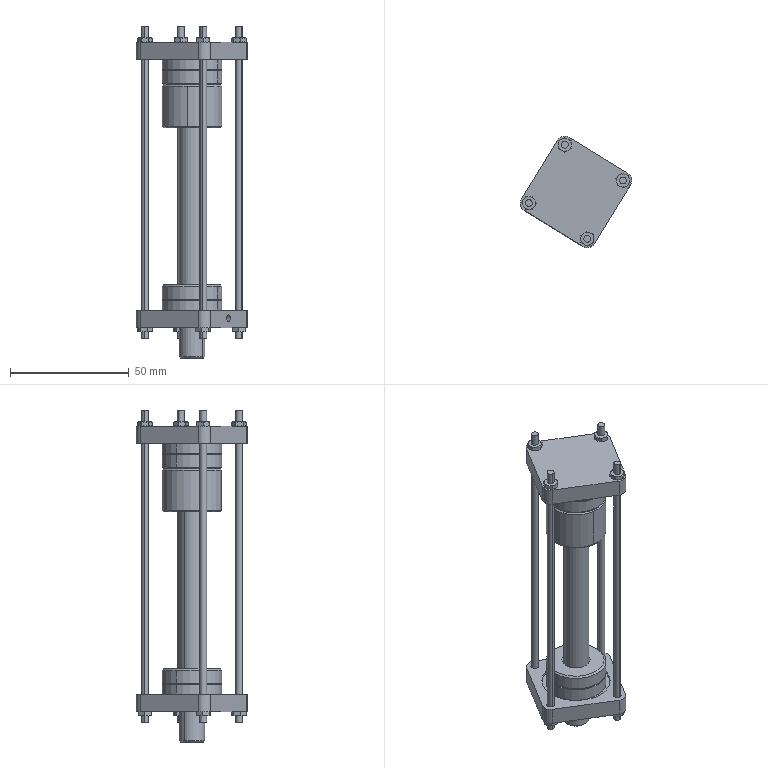Part | SolidWorks | features CompositeCurve 4 | 17 solids | 324 faces | box 46.813 x 46.813 x 139.8 mm | volume 47069 mm3 | cone 126 | plane 110 | cylinder 88 | commonest cylinder face diameters 2.459 x16 3.24 x16 7.2 x12 25.2 x10 2.88 x8 10.8 x8